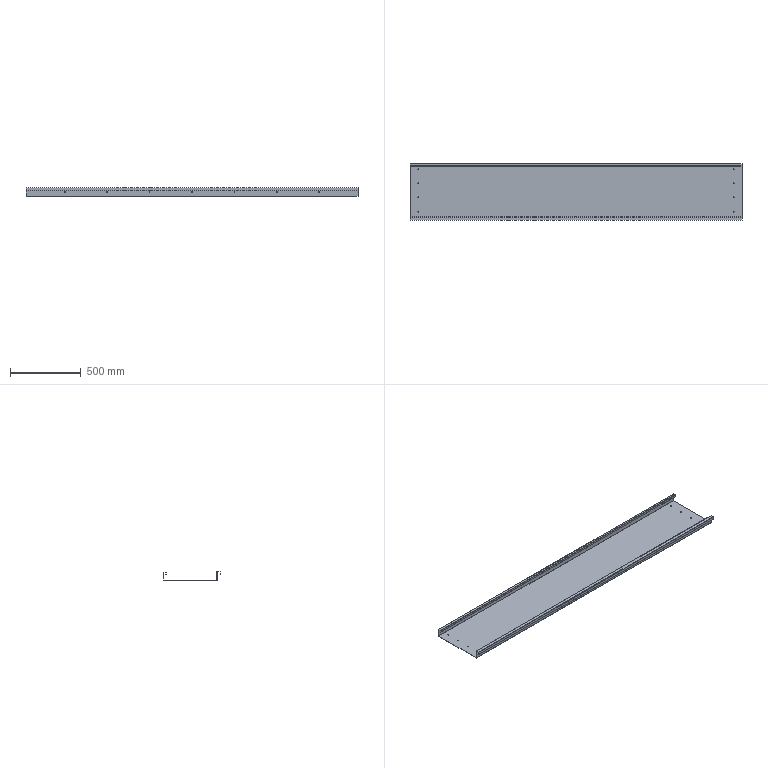Part | STEP file | TS-S16 | 1 solid | 98 faces | box 2350 x 403 x 62 mm | volume 2649119 mm3 | cylinder 56 | plane 42 | commonest cylinder face diameters 5.4 x28 7 x16 0.4 x6 4.4 x6